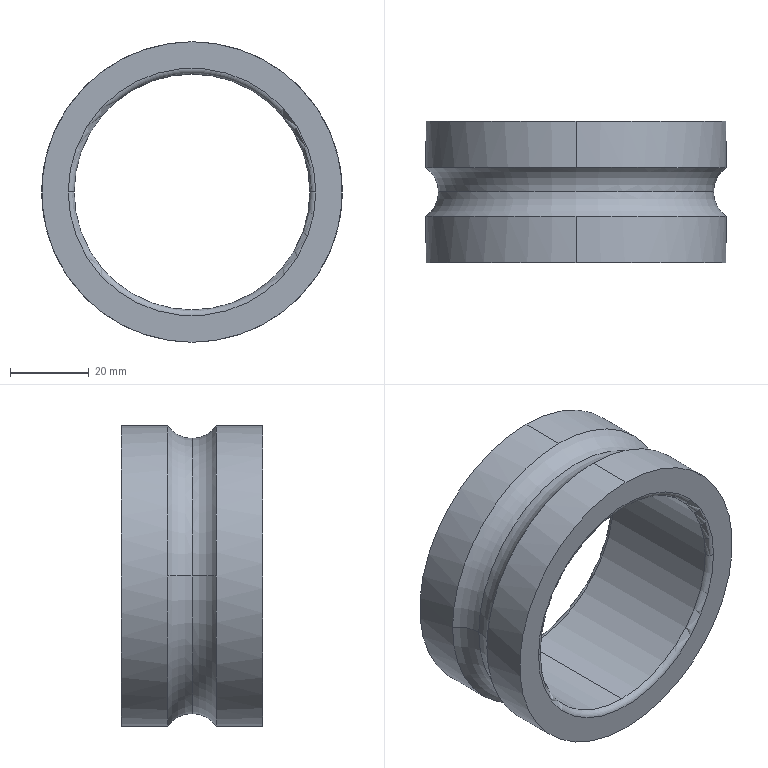Part | SolidWorks | features BaseBody 1 | 1 solid | 16 faces | box 76.5 x 36 x 76.5 mm | volume 56953 mm3 | torus 8 | cylinder 6 | plane 2 | commonest cylinder face diameters 76.5 x4 60 x2
STEP:
#1=CARTESIAN_POINT('',(-2101.45,1017.569,-1577.624));
#2=VERTEX_POINT('',#1);
#3=CARTESIAN_POINT('',(-2164.45,1017.569,-1577.624));
#4=VERTEX_POINT('',#3);
#5=CARTESIAN_POINT('',(-2132.95,1017.569,-1577.624));
#6=DIRECTION('',(0.,-1.,0.));
#7=DIRECTION('',(1.,0.,0.));
#8=AXIS2_PLACEMENT_3D('',#5,#6,#7);
#9=CIRCLE('',#8,31.5);
#10=EDGE_CURVE('',#2,#4,#9,.T.);
#11=ORIENTED_EDGE('',*,*,#10,.F.);
#12=CARTESIAN_POINT('',(-2132.95,1017.569,-1577.624));
#13=DIRECTION('',(0.,-1.,0.));
#14=DIRECTION('',(-1.,0.,0.));
#15=AXIS2_PLACEMENT_3D('',#12,#13,#14);
#16=CIRCLE('',#15,31.5);
#17=EDGE_CURVE('',#4,#2,#16,.T.);
#18=ORIENTED_EDGE('',*,*,#17,.F.);
#19=EDGE_LOOP('',(#11,#18));
#20=FACE_BOUND('',#19,.T.);
#21=CARTESIAN_POINT('',(-2132.95,1017.569,-1615.874));
#22=VERTEX_POINT('',#21);
#23=CARTESIAN_POINT('',(-2132.95,1017.569,-1539.374));
#24=VERTEX_POINT('',#23);
#25=CARTESIAN_POINT('',(-2132.95,1017.569,-1577.624));
#26=DIRECTION('',(0.,-1.,0.));
#27=DIRECTION('',(0.,0.,-1.));
#28=AXIS2_PLACEMENT_3D('',#25,#26,#27);
#29=CIRCLE('',#28,38.25);
#30=EDGE_CURVE('',#22,#24,#29,.T.);
#31=ORIENTED_EDGE('',*,*,#30,.T.);
#32=CARTESIAN_POINT('',(-2132.95,1017.569,-1577.624));
#33=DIRECTION('',(0.,-1.,0.));
#34=DIRECTION('',(0.,0.,1.));
#35=AXIS2_PLACEMENT_3D('',#32,#33,#34);
#36=CIRCLE('',#35,38.25);
#37=EDGE_CURVE('',#24,#22,#36,.T.);
#38=ORIENTED_EDGE('',*,*,#37,.T.);
#39=EDGE_LOOP('',(#31,#38));
#40=FACE_OUTER_BOUND('',#39,.T.);
#41=CARTESIAN_POINT('',(-2175.025,1017.569,-1535.549));
#42=DIRECTION('',(0.,-1.,0.));
#43=DIRECTION('',(0.,0.,-1.));
#44=AXIS2_PLACEMENT_3D('',#41,#42,#43);
#45=PLANE('',#44);
#46=ADVANCED_FACE('',(#20,#40),#45,.T.);
#47=CARTESIAN_POINT('',(-2162.95,1019.069,-1577.624));
#48=VERTEX_POINT('',#47);
#49=CARTESIAN_POINT('',(-2164.45,1019.069,-1577.624));
#50=DIRECTION('',(0.,0.,-1.));
#51=DIRECTION('',(1.,0.,0.));
#52=AXIS2_PLACEMENT_3D('',#49,#50,#51);
#53=CIRCLE('',#52,1.5);
#54=EDGE_CURVE('',#48,#4,#53,.T.);
#55=ORIENTED_EDGE('',*,*,#54,.T.);
#56=ORIENTED_EDGE('',*,*,#17,.T.);
#57=CARTESIAN_POINT('',(-2102.95,1019.069,-1577.624));
#58=VERTEX_POINT('',#57);
#59=CARTESIAN_POINT('',(-2101.45,1019.069,-1577.624));
#60=DIRECTION('',(0.,0.,-1.));
#61=DIRECTION('',(0.,-1.,0.));
#62=AXIS2_PLACEMENT_3D('',#59,#60,#61);
#63=CIRCLE('',#62,1.5);
#64=EDGE_CURVE('',#2,#58,#63,.T.);
#65=ORIENTED_EDGE('',*,*,#64,.T.);
#66=CARTESIAN_POINT('',(-2132.95,1019.069,-1607.624));
#67=VERTEX_POINT('',#66);
#68=CARTESIAN_POINT('',(-2132.95,1019.069,-1577.624));
#69=DIRECTION('',(0.,1.,0.));
#70=DIRECTION('',(1.,0.,0.));
#71=AXIS2_PLACEMENT_3D('',#68,#69,#70);
#72=CIRCLE('',#71,30.);
#73=EDGE_CURVE('',#58,#67,#72,.T.);
#74=ORIENTED_EDGE('',*,*,#73,.T.);
#75=CARTESIAN_POINT('',(-2132.95,1019.069,-1577.624));
#76=DIRECTION('',(0.,1.,0.));
#77=DIRECTION('',(0.,0.,-1.));
#78=AXIS2_PLACEMENT_3D('',#75,#76,#77);
#79=CIRCLE('',#78,30.);
#80=EDGE_CURVE('',#67,#48,#79,.T.);
#81=ORIENTED_EDGE('',*,*,#80,.T.);
#82=EDGE_LOOP('',(#55,#56,#65,#74,#81));
#83=FACE_OUTER_BOUND('',#82,.T.);
#84=CARTESIAN_POINT('',(-2132.95,1019.069,-1577.624));
#85=DIRECTION('',(0.,1.,0.));
#86=DIRECTION('',(0.9962,0.,0.08716));
#87=AXIS2_PLACEMENT_3D('',#84,#85,#86);
#88=TOROIDAL_SURFACE('',#87,31.5,1.5);
#89=ADVANCED_FACE('',(#83),#88,.T.);
#90=CARTESIAN_POINT('',(-2132.95,1019.069,-1547.624));
#91=VERTEX_POINT('',#90);
#92=CARTESIAN_POINT('',(-2132.95,1052.069,-1547.624));
#93=VERTEX_POINT('',#92);
#94=CARTESIAN_POINT('',(-2132.95,1019.069,-1547.624));
#95=DIRECTION('',(0.,1.,0.));
#96=VECTOR('',#95,1000.);
#97=LINE('',#94,#96);
#98=EDGE_CURVE('',#91,#93,#97,.T.);
#99=ORIENTED_EDGE('',*,*,#98,.T.);
#100=CARTESIAN_POINT('',(-2102.95,1052.069,-1577.624));
#101=VERTEX_POINT('',#100);
#102=CARTESIAN_POINT('',(-2132.95,1052.069,-1577.624));
#103=DIRECTION('',(0.,1.,0.));
#104=DIRECTION('',(0.,0.,1.));
#105=AXIS2_PLACEMENT_3D('',#102,#103,#104);
#106=CIRCLE('',#105,30.);
#107=EDGE_CURVE('',#93,#101,#106,.T.);
#108=ORIENTED_EDGE('',*,*,#107,.T.);
#109=CARTESIAN_POINT('',(-2132.95,1052.069,-1607.624));
#110=VERTEX_POINT('',#109);
#111=CARTESIAN_POINT('',(-2132.95,1052.069,-1577.624));
#112=DIRECTION('',(0.,1.,0.));
#113=DIRECTION('',(1.,0.,0.));
#114=AXIS2_PLACEMENT_3D('',#111,#112,#113);
#115=CIRCLE('',#114,30.);
#116=EDGE_CURVE('',#101,#110,#115,.T.);
#117=ORIENTED_EDGE('',*,*,#116,.T.);
#118=CARTESIAN_POINT('',(-2132.95,1052.069,-1607.624));
#119=DIRECTION('',(0.,-1.,0.));
#120=VECTOR('',#119,1000.);
#121=LINE('',#118,#120);
#122=EDGE_CURVE('',#110,#67,#121,.T.);
#123=ORIENTED_EDGE('',*,*,#122,.T.);
#124=ORIENTED_EDGE('',*,*,#73,.F.);
#125=CARTESIAN_POINT('',(-2132.95,1019.069,-1577.624));
#126=DIRECTION('',(0.,1.,0.));
#127=DIRECTION('',(0.,0.,1.));
#128=AXIS2_PLACEMENT_3D('',#125,#126,#127);
#129=CIRCLE('',#128,30.);
#130=EDGE_CURVE('',#91,#58,#129,.T.);
#131=ORIENTED_EDGE('',*,*,#130,.F.);
#132=EDGE_LOOP('',(#99,#108,#117,#123,#124,#131));
#133=FACE_OUTER_BOUND('',#132,.T.);
#134=CARTESIAN_POINT('',(-2132.95,1053.719,-1577.624));
#135=DIRECTION('',(0.,-1.,0.));
#136=DIRECTION('',(-0.08716,0.,-0.9962));
#137=AXIS2_PLACEMENT_3D('',#134,#135,#136);
#138=CYLINDRICAL_SURFACE('',#137,30.);
#139=ADVANCED_FACE('',(#133),#138,.F.);
#140=CARTESIAN_POINT('',(-2164.45,1053.569,-1577.624));
#141=VERTEX_POINT('',#140);
#142=CARTESIAN_POINT('',(-2162.95,1052.069,-1577.624));
#143=VERTEX_POINT('',#142);
#144=CARTESIAN_POINT('',(-2164.45,1052.069,-1577.624));
#145=DIRECTION('',(0.,0.,-1.));
#146=DIRECTION('',(0.,1.,0.));
#147=AXIS2_PLACEMENT_3D('',#144,#145,#146);
#148=CIRCLE('',#147,1.5);
#149=EDGE_CURVE('',#141,#143,#148,.T.);
#150=ORIENTED_EDGE('',*,*,#149,.T.);
#151=CARTESIAN_POINT('',(-2132.95,1052.069,-1577.624));
#152=DIRECTION('',(0.,1.,0.));
#153=DIRECTION('',(0.,0.,-1.));
#154=AXIS2_PLACEMENT_3D('',#151,#152,#153);
#155=CIRCLE('',#154,30.);
#156=EDGE_CURVE('',#110,#143,#155,.T.);
#157=ORIENTED_EDGE('',*,*,#156,.F.);
#158=ORIENTED_EDGE('',*,*,#116,.F.);
#159=CARTESIAN_POINT('',(-2101.45,1053.569,-1577.624));
#160=VERTEX_POINT('',#159);
#161=CARTESIAN_POINT('',(-2101.45,1052.069,-1577.624));
#162=DIRECTION('',(0.,0.,-1.));
#163=DIRECTION('',(-1.,0.,0.));
#164=AXIS2_PLACEMENT_3D('',#161,#162,#163);
#165=CIRCLE('',#164,1.5);
#166=EDGE_CURVE('',#101,#160,#165,.T.);
#167=ORIENTED_EDGE('',*,*,#166,.T.);
#168=CARTESIAN_POINT('',(-2132.95,1053.569,-1577.624));
#169=DIRECTION('',(0.,1.,0.));
#170=DIRECTION('',(1.,0.,0.));
#171=AXIS2_PLACEMENT_3D('',#168,#169,#170);
#172=CIRCLE('',#171,31.5);
#173=EDGE_CURVE('',#160,#141,#172,.T.);
#174=ORIENTED_EDGE('',*,*,#173,.T.);
#175=EDGE_LOOP('',(#150,#157,#158,#167,#174));
#176=FACE_OUTER_BOUND('',#175,.T.);
#177=CARTESIAN_POINT('',(-2132.95,1052.069,-1577.624));
#178=DIRECTION('',(0.,1.,0.));
#179=DIRECTION('',(0.9962,0.,0.08716));
#180=AXIS2_PLACEMENT_3D('',#177,#178,#179);
#181=TOROIDAL_SURFACE('',#180,31.5,1.5);
#182=ADVANCED_FACE('',(#176),#181,.T.);
#183=CARTESIAN_POINT('',(-2132.95,1053.569,-1577.624));
#184=DIRECTION('',(0.,1.,0.));
#185=DIRECTION('',(0.,0.,1.));
#186=AXIS2_PLACEMENT_3D('',#183,#184,#185);
#187=CIRCLE('',#186,31.5);
#188=EDGE_CURVE('',#141,#160,#187,.T.);
#189=ORIENTED_EDGE('',*,*,#188,.F.);
#190=ORIENTED_EDGE('',*,*,#173,.F.);
#191=EDGE_LOOP('',(#189,#190));
#192=FACE_BOUND('',#191,.T.);
#193=CARTESIAN_POINT('',(-2132.95,1053.569,-1539.374));
#194=VERTEX_POINT('',#193);
#195=CARTESIAN_POINT('',(-2132.95,1053.569,-1615.874));
#196=VERTEX_POINT('',#195);
#197=CARTESIAN_POINT('',(-2132.95,1053.569,-1577.624));
#198=DIRECTION('',(0.,1.,0.));
#199=DIRECTION('',(0.,0.,1.));
#200=AXIS2_PLACEMENT_3D('',#197,#198,#199);
#201=CIRCLE('',#200,38.25);
#202=EDGE_CURVE('',#194,#196,#201,.T.);
#203=ORIENTED_EDGE('',*,*,#202,.T.);
#204=CARTESIAN_POINT('',(-2132.95,1053.569,-1577.624));
#205=DIRECTION('',(0.,1.,0.));
#206=DIRECTION('',(0.,0.,-1.));
#207=AXIS2_PLACEMENT_3D('',#204,#205,#206);
#208=CIRCLE('',#207,38.25);
#209=EDGE_CURVE('',#196,#194,#208,.T.);
#210=ORIENTED_EDGE('',*,*,#209,.T.);
#211=EDGE_LOOP('',(#203,#210));
#212=FACE_OUTER_BOUND('',#211,.T.);
#213=CARTESIAN_POINT('',(-2175.025,1053.569,-1619.699));
#214=DIRECTION('',(0.,1.,0.));
#215=DIRECTION('',(1.,0.,0.));
#216=AXIS2_PLACEMENT_3D('',#213,#214,#215);
#217=PLANE('',#216);
#218=ADVANCED_FACE('',(#192,#212),#217,.T.);
#219=CARTESIAN_POINT('',(-2132.95,1041.748,-1539.374));
#220=VERTEX_POINT('',#219);
#221=CARTESIAN_POINT('',(-2132.95,1041.748,-1539.374));
#222=DIRECTION('',(0.,1.,0.));
#223=VECTOR('',#222,1000.);
#224=LINE('',#221,#223);
#225=EDGE_CURVE('',#220,#194,#224,.T.);
#226=ORIENTED_EDGE('',*,*,#225,.T.);
#227=ORIENTED_EDGE('',*,*,#209,.F.);
#228=CARTESIAN_POINT('',(-2132.95,1041.748,-1615.874));
#229=VERTEX_POINT('',#228);
#230=CARTESIAN_POINT('',(-2132.95,1053.569,-1615.874));
#231=DIRECTION('',(0.,-1.,0.));
#232=VECTOR('',#231,1000.);
#233=LINE('',#230,#232);
#234=EDGE_CURVE('',#196,#229,#233,.T.);
#235=ORIENTED_EDGE('',*,*,#234,.T.);
#236=CARTESIAN_POINT('',(-2171.2,1041.748,-1577.624));
#237=VERTEX_POINT('',#236);
#238=CARTESIAN_POINT('',(-2132.95,1041.748,-1577.624));
#239=DIRECTION('',(0.,1.,0.));
#240=DIRECTION('',(0.,0.,-1.));
#241=AXIS2_PLACEMENT_3D('',#238,#239,#240);
#242=CIRCLE('',#241,38.25);
#243=EDGE_CURVE('',#229,#237,#242,.T.);
#244=ORIENTED_EDGE('',*,*,#243,.T.);
#245=CARTESIAN_POINT('',(-2132.95,1041.748,-1577.624));
#246=DIRECTION('',(0.,1.,0.));
#247=DIRECTION('',(-1.,0.,0.));
#248=AXIS2_PLACEMENT_3D('',#245,#246,#247);
#249=CIRCLE('',#248,38.25);
#250=EDGE_CURVE('',#237,#220,#249,.T.);
#251=ORIENTED_EDGE('',*,*,#250,.T.);
#252=EDGE_LOOP('',(#226,#227,#235,#244,#251));
#253=FACE_OUTER_BOUND('',#252,.T.);
#254=CARTESIAN_POINT('',(-2132.95,1041.157,-1577.624));
#255=DIRECTION('',(0.,-1.,0.));
#256=DIRECTION('',(0.08716,0.,0.9962));
#257=AXIS2_PLACEMENT_3D('',#254,#255,#256);
#258=CYLINDRICAL_SURFACE('',#257,38.25);
#259=ADVANCED_FACE('',(#253),#258,.T.);
#260=CARTESIAN_POINT('',(-2097.95,1035.569,-1577.624));
#261=VERTEX_POINT('',#260);
#262=CARTESIAN_POINT('',(-2167.95,1035.569,-1577.624));
#263=VERTEX_POINT('',#262);
#264=CARTESIAN_POINT('',(-2132.95,1035.569,-1577.624));
#265=DIRECTION('',(0.,-1.,0.));
#266=DIRECTION('',(1.,0.,0.));
#267=AXIS2_PLACEMENT_3D('',#264,#265,#266);
#268=CIRCLE('',#267,35.);
#269=EDGE_CURVE('',#261,#263,#268,.T.);
#270=ORIENTED_EDGE('',*,*,#269,.T.);
#271=CARTESIAN_POINT('',(-2171.2,1029.389,-1577.624));
#272=VERTEX_POINT('',#271);
#273=CARTESIAN_POINT('',(-2175.45,1035.569,-1577.624));
#274=DIRECTION('',(0.,0.,-1.));
#275=DIRECTION('',(1.,0.,0.));
#276=AXIS2_PLACEMENT_3D('',#273,#274,#275);
#277=CIRCLE('',#276,7.5);
#278=EDGE_CURVE('',#263,#272,#277,.T.);
#279=ORIENTED_EDGE('',*,*,#278,.T.);
#280=CARTESIAN_POINT('',(-2132.95,1029.389,-1539.374));
#281=VERTEX_POINT('',#280);
#282=CARTESIAN_POINT('',(-2132.95,1029.389,-1577.624));
#283=DIRECTION('',(0.,1.,0.));
#284=DIRECTION('',(-1.,0.,0.));
#285=AXIS2_PLACEMENT_3D('',#282,#283,#284);
#286=CIRCLE('',#285,38.25);
#287=EDGE_CURVE('',#272,#281,#286,.T.);
#288=ORIENTED_EDGE('',*,*,#287,.T.);
#289=CARTESIAN_POINT('',(-2094.7,1029.389,-1577.624));
#290=VERTEX_POINT('',#289);
#291=CARTESIAN_POINT('',(-2132.95,1029.389,-1577.624));
#292=DIRECTION('',(0.,1.,0.));
#293=DIRECTION('',(0.,0.,1.));
#294=AXIS2_PLACEMENT_3D('',#291,#292,#293);
#295=CIRCLE('',#294,38.25);
#296=EDGE_CURVE('',#281,#290,#295,.T.);
#297=ORIENTED_EDGE('',*,*,#296,.T.);
#298=CARTESIAN_POINT('',(-2090.45,1035.569,-1577.624));
#299=DIRECTION('',(0.,0.,-1.));
#300=DIRECTION('',(-0.5667,-0.8239,0.));
#301=AXIS2_PLACEMENT_3D('',#298,#299,#300);
#302=CIRCLE('',#301,7.5);
#303=EDGE_CURVE('',#290,#261,#302,.T.);
#304=ORIENTED_EDGE('',*,*,#303,.T.);
#305=EDGE_LOOP('',(#270,#279,#288,#297,#304));
#306=FACE_OUTER_BOUND('',#305,.T.);
#307=CARTESIAN_POINT('',(-2132.95,1035.569,-1577.624));
#308=DIRECTION('',(0.,1.,0.));
#309=DIRECTION('',(-0.9962,0.,-0.08716));
#310=AXIS2_PLACEMENT_3D('',#307,#308,#309);
#311=TOROIDAL_SURFACE('',#310,42.5,7.5);
#312=ADVANCED_FACE('',(#306),#311,.F.);
#313=CARTESIAN_POINT('',(-2132.95,1017.569,-1539.374));
#314=DIRECTION('',(0.,1.,0.));
#315=VECTOR('',#314,1000.);
#316=LINE('',#313,#315);
#317=EDGE_CURVE('',#24,#281,#316,.T.);
#318=ORIENTED_EDGE('',*,*,#317,.T.);
#319=ORIENTED_EDGE('',*,*,#287,.F.);
#320=CARTESIAN_POINT('',(-2132.95,1029.389,-1615.874));
#321=VERTEX_POINT('',#320);
#322=CARTESIAN_POINT('',(-2132.95,1029.389,-1577.624));
#323=DIRECTION('',(0.,1.,0.));
#324=DIRECTION('',(0.,0.,-1.));
#325=AXIS2_PLACEMENT_3D('',#322,#323,#324);
#326=CIRCLE('',#325,38.25);
#327=EDGE_CURVE('',#321,#272,#326,.T.);
#328=ORIENTED_EDGE('',*,*,#327,.F.);
#329=CARTESIAN_POINT('',(-2132.95,1029.389,-1615.874));
#330=DIRECTION('',(0.,-1.,0.));
#331=VECTOR('',#330,1000.);
#332=LINE('',#329,#331);
#333=EDGE_CURVE('',#321,#22,#332,.T.);
#334=ORIENTED_EDGE('',*,*,#333,.T.);
#335=ORIENTED_EDGE('',*,*,#37,.F.);
#336=EDGE_LOOP('',(#318,#319,#328,#334,#335));
#337=FACE_OUTER_BOUND('',#336,.T.);
#338=CARTESIAN_POINT('',(-2132.95,1016.977,-1577.624));
#339=DIRECTION('',(0.,-1.,0.));
#340=DIRECTION('',(0.08716,0.,0.9962));
#341=AXIS2_PLACEMENT_3D('',#338,#339,#340);
#342=CYLINDRICAL_SURFACE('',#341,38.25);
#343=ADVANCED_FACE('',(#337),#342,.T.);
#344=ORIENTED_EDGE('',*,*,#317,.F.);
#345=ORIENTED_EDGE('',*,*,#30,.F.);
#346=ORIENTED_EDGE('',*,*,#333,.F.);
#347=CARTESIAN_POINT('',(-2132.95,1029.389,-1577.624));
#348=DIRECTION('',(0.,1.,0.));
#349=DIRECTION('',(1.,0.,0.));
#350=AXIS2_PLACEMENT_3D('',#347,#348,#349);
#351=CIRCLE('',#350,38.25);
#352=EDGE_CURVE('',#290,#321,#351,.T.);
#353=ORIENTED_EDGE('',*,*,#352,.F.);
#354=ORIENTED_EDGE('',*,*,#296,.F.);
#355=EDGE_LOOP('',(#344,#345,#346,#353,#354));
#356=FACE_OUTER_BOUND('',#355,.T.);
#357=CARTESIAN_POINT('',(-2132.95,1016.977,-1577.624));
#358=DIRECTION('',(0.,-1.,0.));
#359=DIRECTION('',(-0.08716,0.,-0.9962));
#360=AXIS2_PLACEMENT_3D('',#357,#358,#359);
#361=CYLINDRICAL_SURFACE('',#360,38.25);
#362=ADVANCED_FACE('',(#356),#361,.T.);
#363=CARTESIAN_POINT('',(-2132.95,1035.569,-1577.624));
#364=DIRECTION('',(0.,-1.,0.));
#365=DIRECTION('',(-1.,0.,0.));
#366=AXIS2_PLACEMENT_3D('',#363,#364,#365);
#367=CIRCLE('',#366,35.);
#368=EDGE_CURVE('',#263,#261,#367,.T.);
#369=ORIENTED_EDGE('',*,*,#368,.T.);
#370=ORIENTED_EDGE('',*,*,#303,.F.);
#371=ORIENTED_EDGE('',*,*,#352,.T.);
#372=ORIENTED_EDGE('',*,*,#327,.T.);
#373=ORIENTED_EDGE('',*,*,#278,.F.);
#374=EDGE_LOOP('',(#369,#370,#371,#372,#373));
#375=FACE_OUTER_BOUND('',#374,.T.);
#376=CARTESIAN_POINT('',(-2132.95,1035.569,-1577.624));
#377=DIRECTION('',(0.,1.,0.));
#378=DIRECTION('',(0.9962,0.,0.08716));
#379=AXIS2_PLACEMENT_3D('',#376,#377,#378);
#380=TOROIDAL_SURFACE('',#379,42.5,7.5);
#381=ADVANCED_FACE('',(#375),#380,.F.);
#382=ORIENTED_EDGE('',*,*,#225,.F.);
#383=CARTESIAN_POINT('',(-2094.7,1041.748,-1577.624));
#384=VERTEX_POINT('',#383);
#385=CARTESIAN_POINT('',(-2132.95,1041.748,-1577.624));
#386=DIRECTION('',(0.,1.,0.));
#387=DIRECTION('',(0.,0.,1.));
#388=AXIS2_PLACEMENT_3D('',#385,#386,#387);
#389=CIRCLE('',#388,38.25);
#390=EDGE_CURVE('',#220,#384,#389,.T.);
#391=ORIENTED_EDGE('',*,*,#390,.T.);
#392=CARTESIAN_POINT('',(-2132.95,1041.748,-1577.624));
#393=DIRECTION('',(0.,1.,0.));
#394=DIRECTION('',(1.,0.,0.));
#395=AXIS2_PLACEMENT_3D('',#392,#393,#394);
#396=CIRCLE('',#395,38.25);
#397=EDGE_CURVE('',#384,#229,#396,.T.);
#398=ORIENTED_EDGE('',*,*,#397,.T.);
#399=ORIENTED_EDGE('',*,*,#234,.F.);
#400=ORIENTED_EDGE('',*,*,#202,.F.);
#401=EDGE_LOOP('',(#382,#391,#398,#399,#400));
#402=FACE_OUTER_BOUND('',#401,.T.);
#403=CARTESIAN_POINT('',(-2132.95,1041.157,-1577.624));
#404=DIRECTION('',(0.,-1.,0.));
#405=DIRECTION('',(-0.08716,0.,-0.9962));
#406=AXIS2_PLACEMENT_3D('',#403,#404,#405);
#407=CYLINDRICAL_SURFACE('',#406,38.25);
#408=ADVANCED_FACE('',(#402),#407,.T.);
#409=ORIENTED_EDGE('',*,*,#149,.F.);
#410=ORIENTED_EDGE('',*,*,#188,.T.);
#411=ORIENTED_EDGE('',*,*,#166,.F.);
#412=ORIENTED_EDGE('',*,*,#107,.F.);
#413=CARTESIAN_POINT('',(-2132.95,1052.069,-1577.624));
#414=DIRECTION('',(0.,1.,0.));
#415=DIRECTION('',(-1.,0.,0.));
#416=AXIS2_PLACEMENT_3D('',#413,#414,#415);
#417=CIRCLE('',#416,30.);
#418=EDGE_CURVE('',#143,#93,#417,.T.);
#419=ORIENTED_EDGE('',*,*,#418,.F.);
#420=EDGE_LOOP('',(#409,#410,#411,#412,#419));
#421=FACE_OUTER_BOUND('',#420,.T.);
#422=CARTESIAN_POINT('',(-2132.95,1052.069,-1577.624));
#423=DIRECTION('',(0.,1.,0.));
#424=DIRECTION('',(-0.9962,0.,-0.08716));
#425=AXIS2_PLACEMENT_3D('',#422,#423,#424);
#426=TOROIDAL_SURFACE('',#425,31.5,1.5);
#427=ADVANCED_FACE('',(#421),#426,.T.);
#428=ORIENTED_EDGE('',*,*,#98,.F.);
#429=CARTESIAN_POINT('',(-2132.95,1019.069,-1577.624));
#430=DIRECTION('',(0.,1.,0.));
#431=DIRECTION('',(-1.,0.,0.));
#432=AXIS2_PLACEMENT_3D('',#429,#430,#431);
#433=CIRCLE('',#432,30.);
#434=EDGE_CURVE('',#48,#91,#433,.T.);
#435=ORIENTED_EDGE('',*,*,#434,.F.);
#436=ORIENTED_EDGE('',*,*,#80,.F.);
#437=ORIENTED_EDGE('',*,*,#122,.F.);
#438=ORIENTED_EDGE('',*,*,#156,.T.);
#439=ORIENTED_EDGE('',*,*,#418,.T.);
#440=EDGE_LOOP('',(#428,#435,#436,#437,#438,#439));
#441=FACE_OUTER_BOUND('',#440,.T.);
#442=CARTESIAN_POINT('',(-2132.95,1053.719,-1577.624));
#443=DIRECTION('',(0.,-1.,0.));
#444=DIRECTION('',(0.08716,0.,0.9962));
#445=AXIS2_PLACEMENT_3D('',#442,#443,#444);
#446=CYLINDRICAL_SURFACE('',#445,30.);
#447=ADVANCED_FACE('',(#441),#446,.F.);
#448=ORIENTED_EDGE('',*,*,#54,.F.);
#449=ORIENTED_EDGE('',*,*,#434,.T.);
#450=ORIENTED_EDGE('',*,*,#130,.T.);
#451=ORIENTED_EDGE('',*,*,#64,.F.);
#452=ORIENTED_EDGE('',*,*,#10,.T.);
#453=EDGE_LOOP('',(#448,#449,#450,#451,#452));
#454=FACE_OUTER_BOUND('',#453,.T.);
#455=CARTESIAN_POINT('',(-2132.95,1019.069,-1577.624));
#456=DIRECTION('',(0.,1.,0.));
#457=DIRECTION('',(-0.9962,0.,-0.08716));
#458=AXIS2_PLACEMENT_3D('',#455,#456,#457);
#459=TOROIDAL_SURFACE('',#458,31.5,1.5);
#460=ADVANCED_FACE('',(#454),#459,.T.);
#461=ORIENTED_EDGE('',*,*,#368,.F.);
#462=CARTESIAN_POINT('',(-2175.45,1035.569,-1577.624));
#463=DIRECTION('',(0.,0.,-1.));
#464=DIRECTION('',(0.5667,0.8239,0.));
#465=AXIS2_PLACEMENT_3D('',#462,#463,#464);
#466=CIRCLE('',#465,7.5);
#467=EDGE_CURVE('',#237,#263,#466,.T.);
#468=ORIENTED_EDGE('',*,*,#467,.F.);
#469=ORIENTED_EDGE('',*,*,#243,.F.);
#470=ORIENTED_EDGE('',*,*,#397,.F.);
#471=CARTESIAN_POINT('',(-2090.45,1035.569,-1577.624));
#472=DIRECTION('',(0.,0.,-1.));
#473=DIRECTION('',(-1.,0.,0.));
#474=AXIS2_PLACEMENT_3D('',#471,#472,#473);
#475=CIRCLE('',#474,7.5);
#476=EDGE_CURVE('',#261,#384,#475,.T.);
#477=ORIENTED_EDGE('',*,*,#476,.F.);
#478=EDGE_LOOP('',(#461,#468,#469,#470,#477));
#479=FACE_OUTER_BOUND('',#478,.T.);
#480=CARTESIAN_POINT('',(-2132.95,1035.569,-1577.624));
#481=DIRECTION('',(0.,1.,0.));
#482=DIRECTION('',(0.9962,0.,0.08716));
#483=AXIS2_PLACEMENT_3D('',#480,#481,#482);
#484=TOROIDAL_SURFACE('',#483,42.5,7.5);
#485=ADVANCED_FACE('',(#479),#484,.F.);
#486=ORIENTED_EDGE('',*,*,#269,.F.);
#487=ORIENTED_EDGE('',*,*,#476,.T.);
#488=ORIENTED_EDGE('',*,*,#390,.F.);
#489=ORIENTED_EDGE('',*,*,#250,.F.);
#490=ORIENTED_EDGE('',*,*,#467,.T.);
#491=EDGE_LOOP('',(#486,#487,#488,#489,#490));
#492=FACE_OUTER_BOUND('',#491,.T.);
#493=CARTESIAN_POINT('',(-2132.95,1035.569,-1577.624));
#494=DIRECTION('',(0.,1.,0.));
#495=DIRECTION('',(-0.9962,0.,-0.08716));
#496=AXIS2_PLACEMENT_3D('',#493,#494,#495);
#497=TOROIDAL_SURFACE('',#496,42.5,7.5);
#498=ADVANCED_FACE('',(#492),#497,.F.);
#499=CLOSED_SHELL('',(#46,#89,#139,#182,#218,#259,#312,#343,#362,#381,#408,#427,#447,#460,#485,#498));
#500=MANIFOLD_SOLID_BREP('',#499);
#501=CARTESIAN_POINT('',(0.,0.,0.));
#502=DIRECTION('',(0.,0.,1.));
#503=DIRECTION('',(1.,0.,0.));
#504=AXIS2_PLACEMENT_3D('',#501,#502,#503);
#505=(LENGTH_UNIT()NAMED_UNIT(*)SI_UNIT(.MILLI.,.METRE.));
#506=UNCERTAINTY_MEASURE_WITH_UNIT(LENGTH_MEASURE(0.00001),#505,'','');
#507=(NAMED_UNIT(*)PLANE_ANGLE_UNIT()SI_UNIT($,.RADIAN.));
#508=(NAMED_UNIT(*)SI_UNIT($,.STERADIAN.)SOLID_ANGLE_UNIT());
#509=(GEOMETRIC_REPRESENTATION_CONTEXT(3)GLOBAL_UNCERTAINTY_ASSIGNED_CONTEXT((#506))GLOBAL_UNIT_ASSIGNED_CONTEXT((#505,#507,#508))REPRESENTATION_CONTEXT('',''));
#510=ADVANCED_BREP_SHAPE_REPRESENTATION('',(#500,#504),#509);